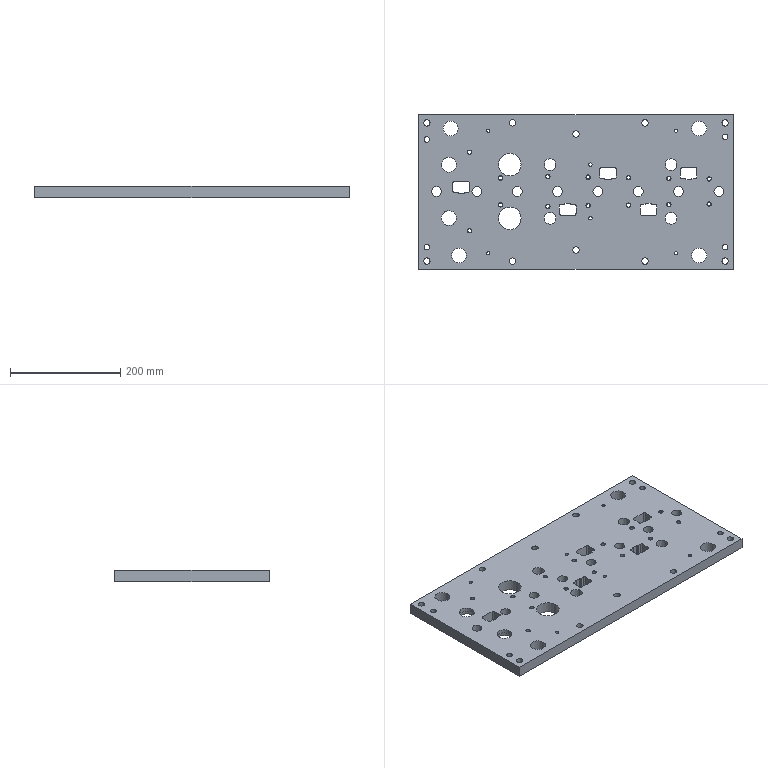Part | NX | features LB-5 2 | 1 solid | 162 faces | box 570 x 280 x 20 mm | volume 2870260 mm3 | cylinder 96 | plane 48 | cone 18 | commonest cylinder face diameters 6 x22 1 x20 6.8 x14 11.5 x10 18.003 x8 27 x6